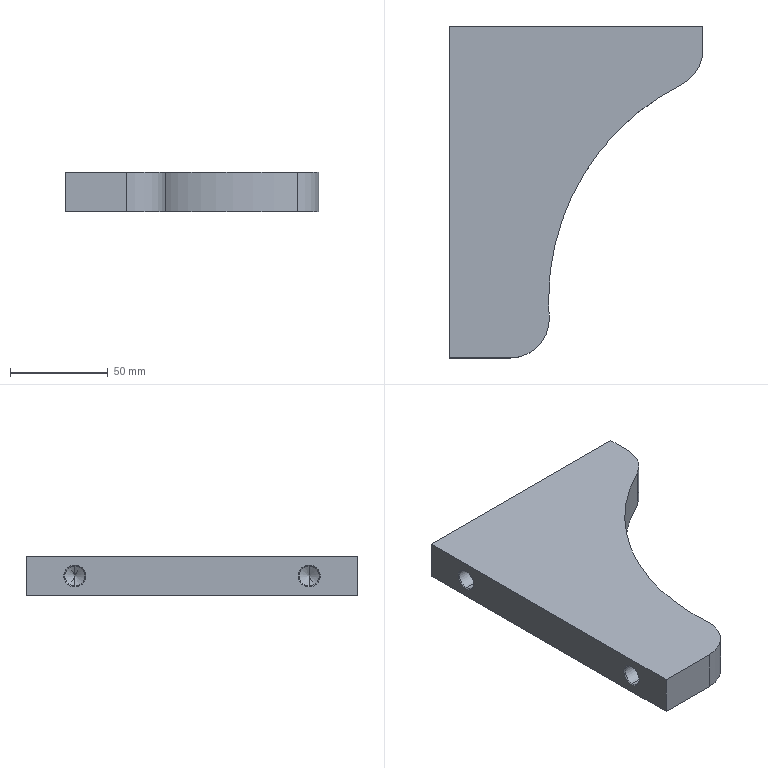Part | STEP file | Driven chain press plate 1 | 1 solid | 22 faces | box 130 x 170 x 20 mm | volume 254830 mm3 | cone 8 | cylinder 8 | plane 6 | commonest cylinder face diameters 10.2 x4 40 x2 246 x2